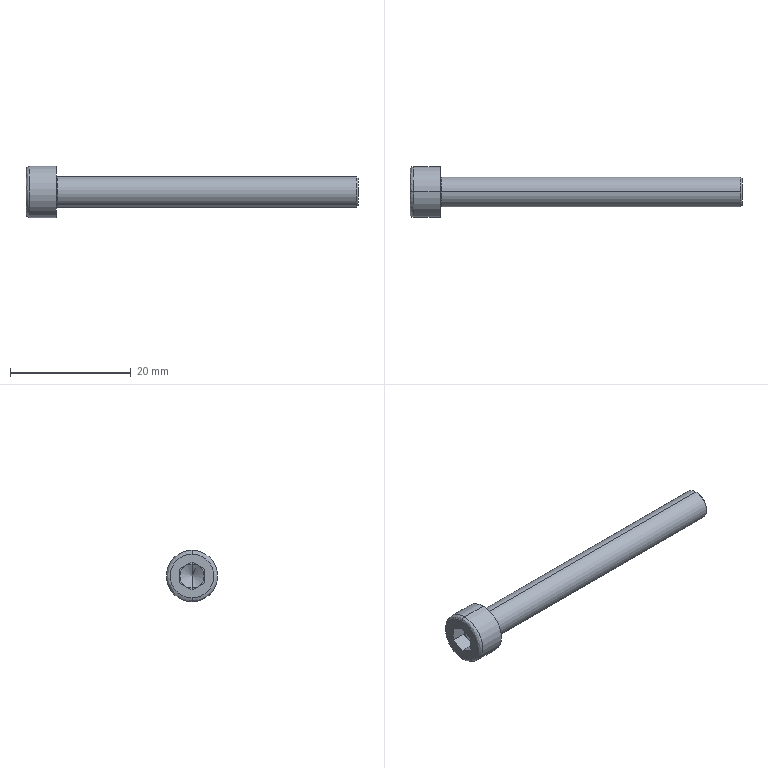Part | SolidWorks | features BaseBody 1 | 1 solid | 27 faces | box 55 x 8.5 x 8.5 mm | volume 1224 mm3 | plane 15 | spline 4 | cylinder 4 | cone 4 | commonest cylinder face diameters 5 x2 8.5 x2
STEP:
#1=CARTESIAN_POINT('',(5.,0.,2.7));
#2=VERTEX_POINT('',#1);
#3=CARTESIAN_POINT('',(5.,0.,-2.7));
#4=VERTEX_POINT('',#3);
#5=CARTESIAN_POINT('',(5.,0.,2.7));
#6=CARTESIAN_POINT('',(5.,0.1716,2.7));
#7=CARTESIAN_POINT('',(5.,0.4245,2.676));
#8=CARTESIAN_POINT('',(5.,0.7118,2.607));
#9=CARTESIAN_POINT('',(5.,0.8535,2.562));
#10=CARTESIAN_POINT('',(5.,0.9138,2.541));
#11=CARTESIAN_POINT('',(5.,0.9539,2.526));
#12=CARTESIAN_POINT('',(5.,0.9722,2.519));
#13=CARTESIAN_POINT('',(5.,1.34,2.373));
#14=CARTESIAN_POINT('',(5.,1.646,2.172));
#15=CARTESIAN_POINT('',(5.,2.041,1.778));
#16=CARTESIAN_POINT('',(5.,2.215,1.564));
#17=CARTESIAN_POINT('',(5.,2.376,1.288));
#18=CARTESIAN_POINT('',(5.,2.447,1.143));
#19=CARTESIAN_POINT('',(5.,2.475,1.08));
#20=CARTESIAN_POINT('',(5.,2.493,1.037));
#21=CARTESIAN_POINT('',(5.,2.503,1.014));
#22=CARTESIAN_POINT('',(5.,2.637,0.675));
#23=CARTESIAN_POINT('',(5.,2.7,0.343));
#24=CARTESIAN_POINT('',(5.,2.7,-0.1715));
#25=CARTESIAN_POINT('',(5.,2.676,-0.4243));
#26=CARTESIAN_POINT('',(5.,2.607,-0.7117));
#27=CARTESIAN_POINT('',(5.,2.562,-0.8534));
#28=CARTESIAN_POINT('',(5.,2.541,-0.9137));
#29=CARTESIAN_POINT('',(5.,2.526,-0.9539));
#30=CARTESIAN_POINT('',(5.,2.519,-0.9722));
#31=CARTESIAN_POINT('',(5.,2.373,-1.34));
#32=CARTESIAN_POINT('',(5.,2.172,-1.646));
#33=CARTESIAN_POINT('',(5.,1.778,-2.041));
#34=CARTESIAN_POINT('',(5.,1.564,-2.215));
#35=CARTESIAN_POINT('',(5.,1.288,-2.376));
#36=CARTESIAN_POINT('',(5.,1.143,-2.447));
#37=CARTESIAN_POINT('',(5.,1.08,-2.475));
#38=CARTESIAN_POINT('',(5.,1.037,-2.493));
#39=CARTESIAN_POINT('',(5.,1.014,-2.503));
#40=CARTESIAN_POINT('',(5.,0.6748,-2.637));
#41=CARTESIAN_POINT('',(5.,0.3435,-2.7));
#42=CARTESIAN_POINT('',(5.,0.,-2.7));
#43=B_SPLINE_CURVE_WITH_KNOTS('',3,(#5,#6,#7,#8,#9,#10,#11,#12,#13,#14,#15,#16,#17,#18,#19,#20,#21,#22,#23,#24,#25,#26,#27,#28,#29,#30,#31,#32,#33,#34,#35,#36,#37,#38,#39,#40,#41,#42),.UNSPECIFIED.,.F.,.F.,(4,1,1,1,2,2,2,1,1,1,2,2,2,1,1,1,2,2,2,1,1,1,2,2,4),(0.,0.0625,0.09375,0.1094,0.1172,0.125,0.25,0.3125,0.3437,0.3594,0.3672,0.375,0.5,0.5625,0.5937,0.6094,0.6172,0.625,0.75,0.8125,0.8437,0.8594,0.8672,0.875,1.),.UNSPECIFIED.);
#44=EDGE_CURVE('',#2,#4,#43,.T.);
#45=ORIENTED_EDGE('',*,*,#44,.F.);
#46=CARTESIAN_POINT('',(5.2,0.,2.5));
#47=VERTEX_POINT('',#46);
#48=CARTESIAN_POINT('',(5.2,0.,2.7));
#49=DIRECTION('',(0.,-1.,0.));
#50=DIRECTION('',(0.,0.,1.));
#51=AXIS2_PLACEMENT_3D('',#48,#49,#50);
#52=CIRCLE('',#51,0.2);
#53=EDGE_CURVE('',#2,#47,#52,.T.);
#54=ORIENTED_EDGE('',*,*,#53,.T.);
#55=CARTESIAN_POINT('',(5.2,0.,-2.5));
#56=VERTEX_POINT('',#55);
#57=CARTESIAN_POINT('',(5.2,0.,0.));
#58=DIRECTION('',(1.,0.,0.));
#59=DIRECTION('',(0.,0.,1.));
#60=AXIS2_PLACEMENT_3D('',#57,#58,#59);
#61=CIRCLE('',#60,2.5);
#62=EDGE_CURVE('',#56,#47,#61,.T.);
#63=ORIENTED_EDGE('',*,*,#62,.F.);
#64=CARTESIAN_POINT('',(5.2,0.,-2.7));
#65=DIRECTION('',(0.,1.,0.));
#66=DIRECTION('',(0.,0.,-1.));
#67=AXIS2_PLACEMENT_3D('',#64,#65,#66);
#68=CIRCLE('',#67,0.2);
#69=EDGE_CURVE('',#4,#56,#68,.T.);
#70=ORIENTED_EDGE('',*,*,#69,.F.);
#71=EDGE_LOOP('',(#45,#54,#63,#70));
#72=FACE_OUTER_BOUND('',#71,.T.);
#73=CARTESIAN_POINT('',(5.,0.,-2.7));
#74=CARTESIAN_POINT('',(5.,5.4,-2.7));
#75=CARTESIAN_POINT('',(5.,5.4,2.7));
#76=CARTESIAN_POINT('',(5.,0.,2.7));
#77=CARTESIAN_POINT('',(5.,0.,-2.583));
#78=CARTESIAN_POINT('',(5.,5.166,-2.583));
#79=CARTESIAN_POINT('',(5.,5.166,2.583));
#80=CARTESIAN_POINT('',(5.,0.,2.583));
#81=CARTESIAN_POINT('',(5.083,0.,-2.5));
#82=CARTESIAN_POINT('',(5.083,5.,-2.5));
#83=CARTESIAN_POINT('',(5.083,5.,2.5));
#84=CARTESIAN_POINT('',(5.083,0.,2.5));
#85=CARTESIAN_POINT('',(5.2,0.,-2.5));
#86=CARTESIAN_POINT('',(5.2,5.,-2.5));
#87=CARTESIAN_POINT('',(5.2,5.,2.5));
#88=CARTESIAN_POINT('',(5.2,0.,2.5));
#89=(BOUNDED_SURFACE()B_SPLINE_SURFACE(3,3,((#73,#74,#75,#76),(#77,#78,#79,#80),(#81,#82,#83,#84),(#85,#86,#87,#88)),.UNSPECIFIED.,.F.,.F.,.T.)B_SPLINE_SURFACE_WITH_KNOTS((4,4),(4,4),(0.,1.),(0.,1.),.UNSPECIFIED.)GEOMETRIC_REPRESENTATION_ITEM()RATIONAL_B_SPLINE_SURFACE(((1.,0.3333,0.3333,1.),(0.8047,0.2682,0.2682,0.8047),(0.8047,0.2682,0.2682,0.8047),(1.,0.3333,0.3333,1.)))REPRESENTATION_ITEM('')SURFACE());
#90=ADVANCED_FACE('',(#72),#89,.F.);
#91=CARTESIAN_POINT('',(0.625,0.,4.25));
#92=VERTEX_POINT('',#91);
#93=CARTESIAN_POINT('',(0.625,0.,-4.25));
#94=VERTEX_POINT('',#93);
#95=CARTESIAN_POINT('',(0.625,0.,0.));
#96=DIRECTION('',(1.,0.,0.));
#97=DIRECTION('',(0.,0.,1.));
#98=AXIS2_PLACEMENT_3D('',#95,#96,#97);
#99=CIRCLE('',#98,4.25);
#100=EDGE_CURVE('',#92,#94,#99,.T.);
#101=ORIENTED_EDGE('',*,*,#100,.F.);
#102=CARTESIAN_POINT('',(0.,0.,3.625));
#103=VERTEX_POINT('',#102);
#104=CARTESIAN_POINT('',(0.625,0.,3.625));
#105=DIRECTION('',(0.,-1.,0.));
#106=DIRECTION('',(0.,0.,1.));
#107=AXIS2_PLACEMENT_3D('',#104,#105,#106);
#108=CIRCLE('',#107,0.625);
#109=EDGE_CURVE('',#92,#103,#108,.T.);
#110=ORIENTED_EDGE('',*,*,#109,.T.);
#111=CARTESIAN_POINT('',(0.,0.,-3.625));
#112=VERTEX_POINT('',#111);
#113=CARTESIAN_POINT('',(0.,0.,3.625));
#114=CARTESIAN_POINT('',(0.,-7.25,3.625));
#115=CARTESIAN_POINT('',(0.,-7.25,-3.625));
#116=CARTESIAN_POINT('',(0.,0.,-3.625));
#117=(BOUNDED_CURVE()B_SPLINE_CURVE(3,(#113,#114,#115,#116),.UNSPECIFIED.,.F.,.F.)B_SPLINE_CURVE_WITH_KNOTS((4,4),(0.,1.),.UNSPECIFIED.)CURVE()GEOMETRIC_REPRESENTATION_ITEM()RATIONAL_B_SPLINE_CURVE((1.,0.3333,0.3333,1.))REPRESENTATION_ITEM(''));
#118=EDGE_CURVE('',#103,#112,#117,.T.);
#119=ORIENTED_EDGE('',*,*,#118,.T.);
#120=CARTESIAN_POINT('',(0.625,0.,-3.625));
#121=DIRECTION('',(0.,1.,0.));
#122=DIRECTION('',(0.,0.,-1.));
#123=AXIS2_PLACEMENT_3D('',#120,#121,#122);
#124=CIRCLE('',#123,0.625);
#125=EDGE_CURVE('',#94,#112,#124,.T.);
#126=ORIENTED_EDGE('',*,*,#125,.F.);
#127=EDGE_LOOP('',(#101,#110,#119,#126));
#128=FACE_OUTER_BOUND('',#127,.T.);
#129=CARTESIAN_POINT('',(0.625,0.,4.25));
#130=CARTESIAN_POINT('',(0.625,-8.5,4.25));
#131=CARTESIAN_POINT('',(0.625,-8.5,-4.25));
#132=CARTESIAN_POINT('',(0.625,0.,-4.25));
#133=CARTESIAN_POINT('',(0.2589,0.,4.25));
#134=CARTESIAN_POINT('',(0.2589,-8.5,4.25));
#135=CARTESIAN_POINT('',(0.2589,-8.5,-4.25));
#136=CARTESIAN_POINT('',(0.2589,0.,-4.25));
#137=CARTESIAN_POINT('',(0.,0.,3.991));
#138=CARTESIAN_POINT('',(0.,-7.982,3.991));
#139=CARTESIAN_POINT('',(0.,-7.982,-3.991));
#140=CARTESIAN_POINT('',(0.,0.,-3.991));
#141=CARTESIAN_POINT('',(0.,0.,3.625));
#142=CARTESIAN_POINT('',(0.,-7.25,3.625));
#143=CARTESIAN_POINT('',(0.,-7.25,-3.625));
#144=CARTESIAN_POINT('',(0.,0.,-3.625));
#145=(BOUNDED_SURFACE()B_SPLINE_SURFACE(3,3,((#129,#130,#131,#132),(#133,#134,#135,#136),(#137,#138,#139,#140),(#141,#142,#143,#144)),.UNSPECIFIED.,.F.,.F.,.F.)B_SPLINE_SURFACE_WITH_KNOTS((4,4),(4,4),(0.,1.),(0.,1.),.UNSPECIFIED.)GEOMETRIC_REPRESENTATION_ITEM()RATIONAL_B_SPLINE_SURFACE(((1.,0.3333,0.3333,1.),(0.8047,0.2682,0.2682,0.8047),(0.8047,0.2682,0.2682,0.8047),(1.,0.3333,0.3333,1.)))REPRESENTATION_ITEM('')SURFACE());
#146=ADVANCED_FACE('',(#128),#145,.T.);
#147=CARTESIAN_POINT('',(54.8,0.,2.5));
#148=VERTEX_POINT('',#147);
#149=CARTESIAN_POINT('',(54.8,0.,-2.5));
#150=VERTEX_POINT('',#149);
#151=CARTESIAN_POINT('',(54.8,0.,0.));
#152=DIRECTION('',(-1.,0.,0.));
#153=DIRECTION('',(0.,0.,1.));
#154=AXIS2_PLACEMENT_3D('',#151,#152,#153);
#155=CIRCLE('',#154,2.5);
#156=EDGE_CURVE('',#148,#150,#155,.T.);
#157=ORIENTED_EDGE('',*,*,#156,.T.);
#158=CARTESIAN_POINT('',(55.,0.,-2.5));
#159=DIRECTION('',(-1.,0.,0.));
#160=VECTOR('',#159,1000.);
#161=LINE('',#158,#160);
#162=EDGE_CURVE('',#150,#56,#161,.T.);
#163=ORIENTED_EDGE('',*,*,#162,.T.);
#164=ORIENTED_EDGE('',*,*,#62,.T.);
#165=CARTESIAN_POINT('',(55.,0.,2.5));
#166=DIRECTION('',(-1.,0.,0.));
#167=VECTOR('',#166,1000.);
#168=LINE('',#165,#167);
#169=EDGE_CURVE('',#148,#47,#168,.T.);
#170=ORIENTED_EDGE('',*,*,#169,.F.);
#171=EDGE_LOOP('',(#157,#163,#164,#170));
#172=FACE_OUTER_BOUND('',#171,.T.);
#173=CARTESIAN_POINT('',(55.,0.,0.));
#174=DIRECTION('',(-1.,0.,0.));
#175=DIRECTION('',(0.,0.,1.));
#176=AXIS2_PLACEMENT_3D('',#173,#174,#175);
#177=CYLINDRICAL_SURFACE('',#176,2.5);
#178=ADVANCED_FACE('',(#172),#177,.T.);
#179=CARTESIAN_POINT('',(55.,0.,2.3));
#180=VERTEX_POINT('',#179);
#181=CARTESIAN_POINT('',(55.,0.,-2.3));
#182=VERTEX_POINT('',#181);
#183=CARTESIAN_POINT('',(55.,0.,0.));
#184=DIRECTION('',(-1.,0.,0.));
#185=DIRECTION('',(0.,0.,1.));
#186=AXIS2_PLACEMENT_3D('',#183,#184,#185);
#187=CIRCLE('',#186,2.3);
#188=EDGE_CURVE('',#180,#182,#187,.T.);
#189=ORIENTED_EDGE('',*,*,#188,.T.);
#190=CARTESIAN_POINT('',(54.8,0.,-2.5));
#191=DIRECTION('',(-0.7071,0.,-0.7071));
#192=VECTOR('',#191,1000.);
#193=LINE('',#190,#192);
#194=EDGE_CURVE('',#182,#150,#193,.T.);
#195=ORIENTED_EDGE('',*,*,#194,.T.);
#196=ORIENTED_EDGE('',*,*,#156,.F.);
#197=CARTESIAN_POINT('',(54.8,0.,2.5));
#198=DIRECTION('',(-0.7071,0.,0.7071));
#199=VECTOR('',#198,1000.);
#200=LINE('',#197,#199);
#201=EDGE_CURVE('',#180,#148,#200,.T.);
#202=ORIENTED_EDGE('',*,*,#201,.F.);
#203=EDGE_LOOP('',(#189,#195,#196,#202));
#204=FACE_OUTER_BOUND('',#203,.T.);
#205=CARTESIAN_POINT('',(54.8,0.,0.));
#206=DIRECTION('',(-1.,0.,0.));
#207=DIRECTION('',(0.,0.,1.));
#208=AXIS2_PLACEMENT_3D('',#205,#206,#207);
#209=CONICAL_SURFACE('',#208,2.5,0.7854);
#210=ADVANCED_FACE('',(#204),#209,.T.);
#211=CARTESIAN_POINT('',(5.,0.,-4.25));
#212=VERTEX_POINT('',#211);
#213=CARTESIAN_POINT('',(5.,0.,4.25));
#214=VERTEX_POINT('',#213);
#215=CARTESIAN_POINT('',(5.,0.,0.));
#216=DIRECTION('',(1.,0.,0.));
#217=DIRECTION('',(0.,0.,1.));
#218=AXIS2_PLACEMENT_3D('',#215,#216,#217);
#219=CIRCLE('',#218,4.25);
#220=EDGE_CURVE('',#212,#214,#219,.T.);
#221=ORIENTED_EDGE('',*,*,#220,.F.);
#222=CARTESIAN_POINT('',(5.,0.,-4.25));
#223=DIRECTION('',(-1.,0.,0.));
#224=VECTOR('',#223,1000.);
#225=LINE('',#222,#224);
#226=EDGE_CURVE('',#212,#94,#225,.T.);
#227=ORIENTED_EDGE('',*,*,#226,.T.);
#228=CARTESIAN_POINT('',(0.625,0.,0.));
#229=DIRECTION('',(1.,0.,0.));
#230=DIRECTION('',(0.,0.,1.));
#231=AXIS2_PLACEMENT_3D('',#228,#229,#230);
#232=CIRCLE('',#231,4.25);
#233=EDGE_CURVE('',#94,#92,#232,.T.);
#234=ORIENTED_EDGE('',*,*,#233,.T.);
#235=CARTESIAN_POINT('',(5.,0.,4.25));
#236=DIRECTION('',(-1.,0.,0.));
#237=VECTOR('',#236,1000.);
#238=LINE('',#235,#237);
#239=EDGE_CURVE('',#214,#92,#238,.T.);
#240=ORIENTED_EDGE('',*,*,#239,.F.);
#241=EDGE_LOOP('',(#221,#227,#234,#240));
#242=FACE_OUTER_BOUND('',#241,.T.);
#243=CARTESIAN_POINT('',(5.,0.,0.));
#244=DIRECTION('',(-1.,0.,0.));
#245=DIRECTION('',(0.,0.,1.));
#246=AXIS2_PLACEMENT_3D('',#243,#244,#245);
#247=CYLINDRICAL_SURFACE('',#246,4.25);
#248=ADVANCED_FACE('',(#242),#247,.T.);
#249=CARTESIAN_POINT('',(3.655,0.,0.));
#250=VERTEX_POINT('',#249);
#251=CARTESIAN_POINT('',(2.5,0.,2.));
#252=VERTEX_POINT('',#251);
#253=CARTESIAN_POINT('',(2.5,0.,2.));
#254=DIRECTION('',(-0.5,0.,0.866));
#255=VECTOR('',#254,1000.);
#256=LINE('',#253,#255);
#257=EDGE_CURVE('',#250,#252,#256,.T.);
#258=ORIENTED_EDGE('',*,*,#257,.F.);
#259=CARTESIAN_POINT('',(2.5,0.,-2.));
#260=VERTEX_POINT('',#259);
#261=CARTESIAN_POINT('',(2.5,0.,-2.));
#262=DIRECTION('',(-0.5,0.,-0.866));
#263=VECTOR('',#262,1000.);
#264=LINE('',#261,#263);
#265=EDGE_CURVE('',#250,#260,#264,.T.);
#266=ORIENTED_EDGE('',*,*,#265,.T.);
#267=CARTESIAN_POINT('',(2.5,-1.,-1.732));
#268=VERTEX_POINT('',#267);
#269=CARTESIAN_POINT('',(2.5,0.,0.));
#270=DIRECTION('',(1.,0.,0.));
#271=DIRECTION('',(0.,0.,1.));
#272=AXIS2_PLACEMENT_3D('',#269,#270,#271);
#273=CIRCLE('',#272,2.);
#274=EDGE_CURVE('',#268,#260,#273,.T.);
#275=ORIENTED_EDGE('',*,*,#274,.F.);
#276=CARTESIAN_POINT('',(2.5,-2.,0.));
#277=VERTEX_POINT('',#276);
#278=CARTESIAN_POINT('',(2.5,0.,0.));
#279=DIRECTION('',(-1.,0.,0.));
#280=DIRECTION('',(0.,0.,1.));
#281=AXIS2_PLACEMENT_3D('',#278,#279,#280);
#282=CIRCLE('',#281,2.);
#283=EDGE_CURVE('',#268,#277,#282,.T.);
#284=ORIENTED_EDGE('',*,*,#283,.T.);
#285=CARTESIAN_POINT('',(2.5,-1.,1.732));
#286=VERTEX_POINT('',#285);
#287=CARTESIAN_POINT('',(2.5,0.,0.));
#288=DIRECTION('',(1.,0.,0.));
#289=DIRECTION('',(0.,0.,1.));
#290=AXIS2_PLACEMENT_3D('',#287,#288,#289);
#291=CIRCLE('',#290,2.);
#292=EDGE_CURVE('',#286,#277,#291,.T.);
#293=ORIENTED_EDGE('',*,*,#292,.F.);
#294=CARTESIAN_POINT('',(2.5,0.,0.));
#295=DIRECTION('',(1.,0.,0.));
#296=DIRECTION('',(0.,0.,1.));
#297=AXIS2_PLACEMENT_3D('',#294,#295,#296);
#298=CIRCLE('',#297,2.);
#299=EDGE_CURVE('',#252,#286,#298,.T.);
#300=ORIENTED_EDGE('',*,*,#299,.F.);
#301=EDGE_LOOP('',(#258,#266,#275,#284,#293,#300));
#302=FACE_OUTER_BOUND('',#301,.T.);
#303=CARTESIAN_POINT('',(2.5,0.,0.));
#304=DIRECTION('',(-1.,0.,0.));
#305=DIRECTION('',(0.,0.,1.));
#306=AXIS2_PLACEMENT_3D('',#303,#304,#305);
#307=CONICAL_SURFACE('',#306,2.,1.047);
#308=ADVANCED_FACE('',(#302),#307,.F.);
#309=ORIENTED_EDGE('',*,*,#162,.F.);
#310=CARTESIAN_POINT('',(54.8,0.,0.));
#311=DIRECTION('',(-1.,0.,0.));
#312=DIRECTION('',(0.,0.,1.));
#313=AXIS2_PLACEMENT_3D('',#310,#311,#312);
#314=CIRCLE('',#313,2.5);
#315=EDGE_CURVE('',#150,#148,#314,.T.);
#316=ORIENTED_EDGE('',*,*,#315,.T.);
#317=ORIENTED_EDGE('',*,*,#169,.T.);
#318=CARTESIAN_POINT('',(5.2,0.,0.));
#319=DIRECTION('',(1.,0.,0.));
#320=DIRECTION('',(0.,0.,1.));
#321=AXIS2_PLACEMENT_3D('',#318,#319,#320);
#322=CIRCLE('',#321,2.5);
#323=EDGE_CURVE('',#47,#56,#322,.T.);
#324=ORIENTED_EDGE('',*,*,#323,.T.);
#325=EDGE_LOOP('',(#309,#316,#317,#324));
#326=FACE_OUTER_BOUND('',#325,.T.);
#327=CARTESIAN_POINT('',(55.,0.,0.));
#328=DIRECTION('',(-1.,0.,0.));
#329=DIRECTION('',(0.,0.,1.));
#330=AXIS2_PLACEMENT_3D('',#327,#328,#329);
#331=CYLINDRICAL_SURFACE('',#330,2.5);
#332=ADVANCED_FACE('',(#326),#331,.T.);
#333=ORIENTED_EDGE('',*,*,#53,.F.);
#334=CARTESIAN_POINT('',(5.,0.,-2.7));
#335=CARTESIAN_POINT('',(5.,-0.1716,-2.7));
#336=CARTESIAN_POINT('',(5.,-0.4245,-2.676));
#337=CARTESIAN_POINT('',(5.,-0.7118,-2.607));
#338=CARTESIAN_POINT('',(5.,-0.8535,-2.562));
#339=CARTESIAN_POINT('',(5.,-0.9138,-2.541));
#340=CARTESIAN_POINT('',(5.,-0.9539,-2.526));
#341=CARTESIAN_POINT('',(5.,-0.9722,-2.519));
#342=CARTESIAN_POINT('',(5.,-1.34,-2.373));
#343=CARTESIAN_POINT('',(5.,-1.646,-2.172));
#344=CARTESIAN_POINT('',(5.,-2.041,-1.778));
#345=CARTESIAN_POINT('',(5.,-2.215,-1.564));
#346=CARTESIAN_POINT('',(5.,-2.376,-1.288));
#347=CARTESIAN_POINT('',(5.,-2.447,-1.143));
#348=CARTESIAN_POINT('',(5.,-2.475,-1.08));
#349=CARTESIAN_POINT('',(5.,-2.493,-1.037));
#350=CARTESIAN_POINT('',(5.,-2.503,-1.014));
#351=CARTESIAN_POINT('',(5.,-2.637,-0.675));
#352=CARTESIAN_POINT('',(5.,-2.7,-0.343));
#353=CARTESIAN_POINT('',(5.,-2.7,0.1715));
#354=CARTESIAN_POINT('',(5.,-2.676,0.4243));
#355=CARTESIAN_POINT('',(5.,-2.607,0.7117));
#356=CARTESIAN_POINT('',(5.,-2.562,0.8534));
#357=CARTESIAN_POINT('',(5.,-2.541,0.9137));
#358=CARTESIAN_POINT('',(5.,-2.526,0.9539));
#359=CARTESIAN_POINT('',(5.,-2.519,0.9722));
#360=CARTESIAN_POINT('',(5.,-2.373,1.34));
#361=CARTESIAN_POINT('',(5.,-2.172,1.646));
#362=CARTESIAN_POINT('',(5.,-1.778,2.041));
#363=CARTESIAN_POINT('',(5.,-1.564,2.215));
#364=CARTESIAN_POINT('',(5.,-1.288,2.376));
#365=CARTESIAN_POINT('',(5.,-1.143,2.447));
#366=CARTESIAN_POINT('',(5.,-1.08,2.475));
#367=CARTESIAN_POINT('',(5.,-1.037,2.493));
#368=CARTESIAN_POINT('',(5.,-1.014,2.503));
#369=CARTESIAN_POINT('',(5.,-0.6748,2.637));
#370=CARTESIAN_POINT('',(5.,-0.3435,2.7));
#371=CARTESIAN_POINT('',(5.,0.,2.7));
#372=B_SPLINE_CURVE_WITH_KNOTS('',3,(#334,#335,#336,#337,#338,#339,#340,#341,#342,#343,#344,#345,#346,#347,#348,#349,#350,#351,#352,#353,#354,#355,#356,#357,#358,#359,#360,#361,#362,#363,#364,#365,#366,#367,#368,#369,#370,#371),.UNSPECIFIED.,.F.,.F.,(4,1,1,1,2,2,2,1,1,1,2,2,2,1,1,1,2,2,2,1,1,1,2,2,4),(0.,0.0625,0.09375,0.1094,0.1172,0.125,0.25,0.3125,0.3437,0.3594,0.3672,0.375,0.5,0.5625,0.5937,0.6094,0.6172,0.625,0.75,0.8125,0.8437,0.8594,0.8672,0.875,1.),.UNSPECIFIED.);
#373=EDGE_CURVE('',#4,#2,#372,.T.);
#374=ORIENTED_EDGE('',*,*,#373,.F.);
#375=ORIENTED_EDGE('',*,*,#69,.T.);
#376=ORIENTED_EDGE('',*,*,#323,.F.);
#377=EDGE_LOOP('',(#333,#374,#375,#376));
#378=FACE_OUTER_BOUND('',#377,.T.);
#379=CARTESIAN_POINT('',(5.,0.,2.7));
#380=CARTESIAN_POINT('',(5.,-5.4,2.7));
#381=CARTESIAN_POINT('',(5.,-5.4,-2.7));
#382=CARTESIAN_POINT('',(5.,0.,-2.7));
#383=CARTESIAN_POINT('',(5.,0.,2.583));
#384=CARTESIAN_POINT('',(5.,-5.166,2.583));
#385=CARTESIAN_POINT('',(5.,-5.166,-2.583));
#386=CARTESIAN_POINT('',(5.,0.,-2.583));
#387=CARTESIAN_POINT('',(5.083,0.,2.5));
#388=CARTESIAN_POINT('',(5.083,-5.,2.5));
#389=CARTESIAN_POINT('',(5.083,-5.,-2.5));
#390=CARTESIAN_POINT('',(5.083,0.,-2.5));
#391=CARTESIAN_POINT('',(5.2,0.,2.5));
#392=CARTESIAN_POINT('',(5.2,-5.,2.5));
#393=CARTESIAN_POINT('',(5.2,-5.,-2.5));
#394=CARTESIAN_POINT('',(5.2,0.,-2.5));
#395=(BOUNDED_SURFACE()B_SPLINE_SURFACE(3,3,((#379,#380,#381,#382),(#383,#384,#385,#386),(#387,#388,#389,#390),(#391,#392,#393,#394)),.UNSPECIFIED.,.F.,.F.,.F.)B_SPLINE_SURFACE_WITH_KNOTS((4,4),(4,4),(0.,1.),(0.,1.),.UNSPECIFIED.)GEOMETRIC_REPRESENTATION_ITEM()RATIONAL_B_SPLINE_SURFACE(((1.,0.3333,0.3333,1.),(0.8047,0.2682,0.2682,0.8047),(0.8047,0.2682,0.2682,0.8047),(1.,0.3333,0.3333,1.)))REPRESENTATION_ITEM('')SURFACE());
#396=ADVANCED_FACE('',(#378),#395,.F.);
#397=ORIENTED_EDGE('',*,*,#194,.F.);
#398=CARTESIAN_POINT('',(55.,0.,0.));
#399=DIRECTION('',(-1.,0.,0.));
#400=DIRECTION('',(0.,0.,1.));
#401=AXIS2_PLACEMENT_3D('',#398,#399,#400);
#402=CIRCLE('',#401,2.3);
#403=EDGE_CURVE('',#182,#180,#402,.T.);
#404=ORIENTED_EDGE('',*,*,#403,.T.);
#405=ORIENTED_EDGE('',*,*,#201,.T.);
#406=ORIENTED_EDGE('',*,*,#315,.F.);
#407=EDGE_LOOP('',(#397,#404,#405,#406));
#408=FACE_OUTER_BOUND('',#407,.T.);
#409=CARTESIAN_POINT('',(54.8,0.,0.));
#410=DIRECTION('',(-1.,0.,0.));
#411=DIRECTION('',(0.,0.,1.));
#412=AXIS2_PLACEMENT_3D('',#409,#410,#411);
#413=CONICAL_SURFACE('',#412,2.5,0.7854);
#414=ADVANCED_FACE('',(#408),#413,.T.);
#415=CARTESIAN_POINT('',(5.,0.,0.));
#416=DIRECTION('',(1.,0.,0.));
#417=DIRECTION('',(0.,0.,1.));
#418=AXIS2_PLACEMENT_3D('',#415,#416,#417);
#419=CIRCLE('',#418,4.25);
#420=EDGE_CURVE('',#214,#212,#419,.T.);
#421=ORIENTED_EDGE('',*,*,#420,.T.);
#422=ORIENTED_EDGE('',*,*,#220,.T.);
#423=EDGE_LOOP('',(#421,#422));
#424=FACE_OUTER_BOUND('',#423,.T.);
#425=ORIENTED_EDGE('',*,*,#373,.T.);
#426=ORIENTED_EDGE('',*,*,#44,.T.);
#427=EDGE_LOOP('',(#425,#426));
#428=FACE_BOUND('',#427,.T.);
#429=CARTESIAN_POINT('',(5.,0.,0.));
#430=DIRECTION('',(1.,0.,0.));
#431=DIRECTION('',(0.,0.,-1.));
#432=AXIS2_PLACEMENT_3D('',#429,#430,#431);
#433=PLANE('',#432);
#434=ADVANCED_FACE('',(#424,#428),#433,.T.);
#435=ORIENTED_EDGE('',*,*,#188,.F.);
#436=ORIENTED_EDGE('',*,*,#403,.F.);
#437=EDGE_LOOP('',(#435,#436));
#438=FACE_OUTER_BOUND('',#437,.T.);
#439=CARTESIAN_POINT('',(55.,0.,0.));
#440=DIRECTION('',(1.,0.,0.));
#441=DIRECTION('',(0.,0.,-1.));
#442=AXIS2_PLACEMENT_3D('',#439,#440,#441);
#443=PLANE('',#442);
#444=ADVANCED_FACE('',(#438),#443,.T.);
#445=ORIENTED_EDGE('',*,*,#226,.F.);
#446=ORIENTED_EDGE('',*,*,#420,.F.);
#447=ORIENTED_EDGE('',*,*,#239,.T.);
#448=ORIENTED_EDGE('',*,*,#100,.T.);
#449=EDGE_LOOP('',(#445,#446,#447,#448));
#450=FACE_OUTER_BOUND('',#449,.T.);
#451=CARTESIAN_POINT('',(5.,0.,0.));
#452=DIRECTION('',(-1.,0.,0.));
#453=DIRECTION('',(0.,0.,1.));
#454=AXIS2_PLACEMENT_3D('',#451,#452,#453);
#455=CYLINDRICAL_SURFACE('',#454,4.25);
#456=ADVANCED_FACE('',(#450),#455,.T.);
#457=ORIENTED_EDGE('',*,*,#109,.F.);
#458=ORIENTED_EDGE('',*,*,#233,.F.);
#459=ORIENTED_EDGE('',*,*,#125,.T.);
#460=CARTESIAN_POINT('',(0.,0.,-3.625));
#461=CARTESIAN_POINT('',(0.,7.25,-3.625));
#462=CARTESIAN_POINT('',(0.,7.25,3.625));
#463=CARTESIAN_POINT('',(0.,0.,3.625));
#464=(BOUNDED_CURVE()B_SPLINE_CURVE(3,(#460,#461,#462,#463),.UNSPECIFIED.,.F.,.F.)B_SPLINE_CURVE_WITH_KNOTS((4,4),(0.,1.),.UNSPECIFIED.)CURVE()GEOMETRIC_REPRESENTATION_ITEM()RATIONAL_B_SPLINE_CURVE((1.,0.3333,0.3333,1.))REPRESENTATION_ITEM(''));
#465=EDGE_CURVE('',#112,#103,#464,.T.);
#466=ORIENTED_EDGE('',*,*,#465,.T.);
#467=EDGE_LOOP('',(#457,#458,#459,#466));
#468=FACE_OUTER_BOUND('',#467,.T.);
#469=CARTESIAN_POINT('',(0.625,0.,-4.25));
#470=CARTESIAN_POINT('',(0.625,8.5,-4.25));
#471=CARTESIAN_POINT('',(0.625,8.5,4.25));
#472=CARTESIAN_POINT('',(0.625,0.,4.25));
#473=CARTESIAN_POINT('',(0.2589,0.,-4.25));
#474=CARTESIAN_POINT('',(0.2589,8.5,-4.25));
#475=CARTESIAN_POINT('',(0.2589,8.5,4.25));
#476=CARTESIAN_POINT('',(0.2589,0.,4.25));
#477=CARTESIAN_POINT('',(0.,0.,-3.991));
#478=CARTESIAN_POINT('',(0.,7.982,-3.991));
#479=CARTESIAN_POINT('',(0.,7.982,3.991));
#480=CARTESIAN_POINT('',(0.,0.,3.991));
#481=CARTESIAN_POINT('',(0.,0.,-3.625));
#482=CARTESIAN_POINT('',(0.,7.25,-3.625));
#483=CARTESIAN_POINT('',(0.,7.25,3.625));
#484=CARTESIAN_POINT('',(0.,0.,3.625));
#485=(BOUNDED_SURFACE()B_SPLINE_SURFACE(3,3,((#469,#470,#471,#472),(#473,#474,#475,#476),(#477,#478,#479,#480),(#481,#482,#483,#484)),.UNSPECIFIED.,.F.,.F.,.T.)B_SPLINE_SURFACE_WITH_KNOTS((4,4),(4,4),(0.,1.),(0.,1.),.UNSPECIFIED.)GEOMETRIC_REPRESENTATION_ITEM()RATIONAL_B_SPLINE_SURFACE(((1.,0.3333,0.3333,1.),(0.8047,0.2682,0.2682,0.8047),(0.8047,0.2682,0.2682,0.8047),(1.,0.3333,0.3333,1.)))REPRESENTATION_ITEM('')SURFACE());
#486=ADVANCED_FACE('',(#468),#485,.T.);
#487=CARTESIAN_POINT('',(0.,2.,1.155));
#488=VERTEX_POINT('',#487);
#489=CARTESIAN_POINT('',(0.,2.,-1.155));
#490=VERTEX_POINT('',#489);
#491=CARTESIAN_POINT('',(0.,2.,0.));
#492=DIRECTION('',(0.,0.,-1.));
#493=VECTOR('',#492,1000.);
#494=LINE('',#491,#493);
#495=EDGE_CURVE('',#488,#490,#494,.T.);
#496=ORIENTED_EDGE('',*,*,#495,.F.);
#497=CARTESIAN_POINT('',(0.,0.,2.309));
#498=VERTEX_POINT('',#497);
#499=CARTESIAN_POINT('',(0.,0.,2.309));
#500=DIRECTION('',(0.,0.866,-0.5));
#501=VECTOR('',#500,1000.);
#502=LINE('',#499,#501);
#503=EDGE_CURVE('',#498,#488,#502,.T.);
#504=ORIENTED_EDGE('',*,*,#503,.F.);
#505=CARTESIAN_POINT('',(0.,-2.,1.155));
#506=VERTEX_POINT('',#505);
#507=CARTESIAN_POINT('',(0.,-2.,1.155));
#508=DIRECTION('',(0.,0.866,0.5));
#509=VECTOR('',#508,1000.);
#510=LINE('',#507,#509);
#511=EDGE_CURVE('',#506,#498,#510,.T.);
#512=ORIENTED_EDGE('',*,*,#511,.F.);
#513=CARTESIAN_POINT('',(0.,-2.,-1.155));
#514=VERTEX_POINT('',#513);
#515=CARTESIAN_POINT('',(0.,-2.,0.));
#516=DIRECTION('',(0.,0.,1.));
#517=VECTOR('',#516,1000.);
#518=LINE('',#515,#517);
#519=EDGE_CURVE('',#514,#506,#518,.T.);
#520=ORIENTED_EDGE('',*,*,#519,.F.);
#521=CARTESIAN_POINT('',(0.,0.,-2.309));
#522=VERTEX_POINT('',#521);
#523=CARTESIAN_POINT('',(0.,0.,-2.309));
#524=DIRECTION('',(0.,-0.866,0.5));
#525=VECTOR('',#524,1000.);
#526=LINE('',#523,#525);
#527=EDGE_CURVE('',#522,#514,#526,.T.);
#528=ORIENTED_EDGE('',*,*,#527,.F.);
#529=CARTESIAN_POINT('',(0.,2.,-1.155));
#530=DIRECTION('',(0.,-0.866,-0.5));
#531=VECTOR('',#530,1000.);
#532=LINE('',#529,#531);
#533=EDGE_CURVE('',#490,#522,#532,.T.);
#534=ORIENTED_EDGE('',*,*,#533,.F.);
#535=EDGE_LOOP('',(#496,#504,#512,#520,#528,#534));
#536=FACE_BOUND('',#535,.T.);
#537=ORIENTED_EDGE('',*,*,#465,.F.);
#538=ORIENTED_EDGE('',*,*,#118,.F.);
#539=EDGE_LOOP('',(#537,#538));
#540=FACE_OUTER_BOUND('',#539,.T.);
#541=CARTESIAN_POINT('',(0.,0.,0.));
#542=DIRECTION('',(1.,0.,0.));
#543=DIRECTION('',(0.,0.,-1.));
#544=AXIS2_PLACEMENT_3D('',#541,#542,#543);
#545=PLANE('',#544);
#546=ADVANCED_FACE('',(#536,#540),#545,.F.);
#547=CARTESIAN_POINT('',(2.5,0.,-2.309));
#548=VERTEX_POINT('',#547);
#549=CARTESIAN_POINT('',(2.5,0.,-2.309));
#550=DIRECTION('',(1.,0.,0.));
#551=VECTOR('',#550,1000.);
#552=LINE('',#549,#551);
#553=EDGE_CURVE('',#522,#548,#552,.T.);
#554=ORIENTED_EDGE('',*,*,#553,.T.);
#555=CARTESIAN_POINT('',(2.5,1.,-1.732));
#556=VERTEX_POINT('',#555);
#557=CARTESIAN_POINT('',(2.5,0.,-2.309));
#558=DIRECTION('',(0.,0.866,0.5));
#559=VECTOR('',#558,1000.);
#560=LINE('',#557,#559);
#561=EDGE_CURVE('',#548,#556,#560,.T.);
#562=ORIENTED_EDGE('',*,*,#561,.T.);
#563=CARTESIAN_POINT('',(2.5,2.,-1.155));
#564=VERTEX_POINT('',#563);
#565=CARTESIAN_POINT('',(2.5,1.,-1.732));
#566=DIRECTION('',(0.,0.866,0.5));
#567=VECTOR('',#566,1000.);
#568=LINE('',#565,#567);
#569=EDGE_CURVE('',#556,#564,#568,.T.);
#570=ORIENTED_EDGE('',*,*,#569,.T.);
#571=CARTESIAN_POINT('',(2.5,2.,-1.155));
#572=DIRECTION('',(-1.,0.,0.));
#573=VECTOR('',#572,1000.);
#574=LINE('',#571,#573);
#575=EDGE_CURVE('',#564,#490,#574,.T.);
#576=ORIENTED_EDGE('',*,*,#575,.T.);
#577=ORIENTED_EDGE('',*,*,#533,.T.);
#578=EDGE_LOOP('',(#554,#562,#570,#576,#577));
#579=FACE_OUTER_BOUND('',#578,.T.);
#580=CARTESIAN_POINT('',(2.5,0.,-2.309));
#581=DIRECTION('',(0.,-0.5,0.866));
#582=DIRECTION('',(0.,-0.866,-0.5));
#583=AXIS2_PLACEMENT_3D('',#580,#581,#582);
#584=PLANE('',#583);
#585=ADVANCED_FACE('',(#579),#584,.T.);
#586=ORIENTED_EDGE('',*,*,#575,.F.);
#587=CARTESIAN_POINT('',(2.5,2.,0.));
#588=VERTEX_POINT('',#587);
#589=CARTESIAN_POINT('',(2.5,2.,-2.309));
#590=DIRECTION('',(0.,0.,1.));
#591=VECTOR('',#590,1000.);
#592=LINE('',#589,#591);
#593=EDGE_CURVE('',#564,#588,#592,.T.);
#594=ORIENTED_EDGE('',*,*,#593,.T.);
#595=CARTESIAN_POINT('',(2.5,2.,1.155));
#596=VERTEX_POINT('',#595);
#597=CARTESIAN_POINT('',(2.5,2.,-2.309));
#598=DIRECTION('',(0.,0.,1.));
#599=VECTOR('',#598,1000.);
#600=LINE('',#597,#599);
#601=EDGE_CURVE('',#588,#596,#600,.T.);
#602=ORIENTED_EDGE('',*,*,#601,.T.);
#603=CARTESIAN_POINT('',(2.5,2.,1.155));
#604=DIRECTION('',(-1.,0.,0.));
#605=VECTOR('',#604,1000.);
#606=LINE('',#603,#605);
#607=EDGE_CURVE('',#596,#488,#606,.T.);
#608=ORIENTED_EDGE('',*,*,#607,.T.);
#609=ORIENTED_EDGE('',*,*,#495,.T.);
#610=EDGE_LOOP('',(#586,#594,#602,#608,#609));
#611=FACE_OUTER_BOUND('',#610,.T.);
#612=CARTESIAN_POINT('',(2.5,2.,-1.155));
#613=DIRECTION('',(0.,-1.,0.));
#614=DIRECTION('',(0.,0.,-1.));
#615=AXIS2_PLACEMENT_3D('',#612,#613,#614);
#616=PLANE('',#615);
#617=ADVANCED_FACE('',(#611),#616,.T.);
#618=ORIENTED_EDGE('',*,*,#607,.F.);
#619=CARTESIAN_POINT('',(2.5,1.,1.732));
#620=VERTEX_POINT('',#619);
#621=CARTESIAN_POINT('',(2.5,2.,1.155));
#622=DIRECTION('',(0.,-0.866,0.5));
#623=VECTOR('',#622,1000.);
#624=LINE('',#621,#623);
#625=EDGE_CURVE('',#596,#620,#624,.T.);
#626=ORIENTED_EDGE('',*,*,#625,.T.);
#627=CARTESIAN_POINT('',(2.5,0.,2.309));
#628=VERTEX_POINT('',#627);
#629=CARTESIAN_POINT('',(2.5,2.,1.155));
#630=DIRECTION('',(0.,-0.866,0.5));
#631=VECTOR('',#630,1000.);
#632=LINE('',#629,#631);
#633=EDGE_CURVE('',#620,#628,#632,.T.);
#634=ORIENTED_EDGE('',*,*,#633,.T.);
#635=CARTESIAN_POINT('',(2.5,0.,2.309));
#636=DIRECTION('',(-1.,0.,0.));
#637=VECTOR('',#636,1000.);
#638=LINE('',#635,#637);
#639=EDGE_CURVE('',#628,#498,#638,.T.);
#640=ORIENTED_EDGE('',*,*,#639,.T.);
#641=ORIENTED_EDGE('',*,*,#503,.T.);
#642=EDGE_LOOP('',(#618,#626,#634,#640,#641));
#643=FACE_OUTER_BOUND('',#642,.T.);
#644=CARTESIAN_POINT('',(2.5,2.,1.155));
#645=DIRECTION('',(0.,-0.5,-0.866));
#646=DIRECTION('',(0.,0.866,-0.5));
#647=AXIS2_PLACEMENT_3D('',#644,#645,#646);
#648=PLANE('',#647);
#649=ADVANCED_FACE('',(#643),#648,.T.);
#650=ORIENTED_EDGE('',*,*,#639,.F.);
#651=CARTESIAN_POINT('',(2.5,0.,2.309));
#652=DIRECTION('',(0.,-0.866,-0.5));
#653=VECTOR('',#652,1000.);
#654=LINE('',#651,#653);
#655=EDGE_CURVE('',#628,#286,#654,.T.);
#656=ORIENTED_EDGE('',*,*,#655,.T.);
#657=CARTESIAN_POINT('',(2.5,-2.,1.155));
#658=VERTEX_POINT('',#657);
#659=CARTESIAN_POINT('',(2.5,-1.,1.732));
#660=DIRECTION('',(0.,-0.866,-0.5));
#661=VECTOR('',#660,1000.);
#662=LINE('',#659,#661);
#663=EDGE_CURVE('',#286,#658,#662,.T.);
#664=ORIENTED_EDGE('',*,*,#663,.T.);
#665=CARTESIAN_POINT('',(2.5,-2.,1.155));
#666=DIRECTION('',(-1.,0.,0.));
#667=VECTOR('',#666,1000.);
#668=LINE('',#665,#667);
#669=EDGE_CURVE('',#658,#506,#668,.T.);
#670=ORIENTED_EDGE('',*,*,#669,.T.);
#671=ORIENTED_EDGE('',*,*,#511,.T.);
#672=EDGE_LOOP('',(#650,#656,#664,#670,#671));
#673=FACE_OUTER_BOUND('',#672,.T.);
#674=CARTESIAN_POINT('',(2.5,0.,2.309));
#675=DIRECTION('',(0.,0.5,-0.866));
#676=DIRECTION('',(0.,0.866,0.5));
#677=AXIS2_PLACEMENT_3D('',#674,#675,#676);
#678=PLANE('',#677);
#679=ADVANCED_FACE('',(#673),#678,.T.);
#680=ORIENTED_EDGE('',*,*,#669,.F.);
#681=CARTESIAN_POINT('',(2.5,-2.,-2.309));
#682=DIRECTION('',(0.,0.,-1.));
#683=VECTOR('',#682,1000.);
#684=LINE('',#681,#683);
#685=EDGE_CURVE('',#658,#277,#684,.T.);
#686=ORIENTED_EDGE('',*,*,#685,.T.);
#687=CARTESIAN_POINT('',(2.5,-2.,-1.155));
#688=VERTEX_POINT('',#687);
#689=CARTESIAN_POINT('',(2.5,-2.,1.155));
#690=DIRECTION('',(0.,0.,-1.));
#691=VECTOR('',#690,1000.);
#692=LINE('',#689,#691);
#693=EDGE_CURVE('',#277,#688,#692,.T.);
#694=ORIENTED_EDGE('',*,*,#693,.T.);
#695=CARTESIAN_POINT('',(2.5,-2.,-1.155));
#696=DIRECTION('',(-1.,0.,0.));
#697=VECTOR('',#696,1000.);
#698=LINE('',#695,#697);
#699=EDGE_CURVE('',#688,#514,#698,.T.);
#700=ORIENTED_EDGE('',*,*,#699,.T.);
#701=ORIENTED_EDGE('',*,*,#519,.T.);
#702=EDGE_LOOP('',(#680,#686,#694,#700,#701));
#703=FACE_OUTER_BOUND('',#702,.T.);
#704=CARTESIAN_POINT('',(2.5,-2.,1.155));
#705=DIRECTION('',(0.,1.,0.));
#706=DIRECTION('',(0.,0.,1.));
#707=AXIS2_PLACEMENT_3D('',#704,#705,#706);
#708=PLANE('',#707);
#709=ADVANCED_FACE('',(#703),#708,.T.);
#710=ORIENTED_EDGE('',*,*,#699,.F.);
#711=CARTESIAN_POINT('',(2.5,-2.,-1.155));
#712=DIRECTION('',(0.,0.866,-0.5));
#713=VECTOR('',#712,1000.);
#714=LINE('',#711,#713);
#715=EDGE_CURVE('',#688,#268,#714,.T.);
#716=ORIENTED_EDGE('',*,*,#715,.T.);
#717=CARTESIAN_POINT('',(2.5,-2.,-1.155));
#718=DIRECTION('',(0.,0.866,-0.5));
#719=VECTOR('',#718,1000.);
#720=LINE('',#717,#719);
#721=EDGE_CURVE('',#268,#548,#720,.T.);
#722=ORIENTED_EDGE('',*,*,#721,.T.);
#723=ORIENTED_EDGE('',*,*,#553,.F.);
#724=ORIENTED_EDGE('',*,*,#527,.T.);
#725=EDGE_LOOP('',(#710,#716,#722,#723,#724));
#726=FACE_OUTER_BOUND('',#725,.T.);
#727=CARTESIAN_POINT('',(2.5,-2.,-1.155));
#728=DIRECTION('',(0.,0.5,0.866));
#729=DIRECTION('',(0.,-0.866,0.5));
#730=AXIS2_PLACEMENT_3D('',#727,#728,#729);
#731=PLANE('',#730);
#732=ADVANCED_FACE('',(#726),#731,.T.);
#733=ORIENTED_EDGE('',*,*,#274,.T.);
#734=CARTESIAN_POINT('',(2.5,0.,0.));
#735=DIRECTION('',(1.,0.,0.));
#736=DIRECTION('',(0.,0.,1.));
#737=AXIS2_PLACEMENT_3D('',#734,#735,#736);
#738=CIRCLE('',#737,2.);
#739=EDGE_CURVE('',#260,#556,#738,.T.);
#740=ORIENTED_EDGE('',*,*,#739,.T.);
#741=ORIENTED_EDGE('',*,*,#561,.F.);
#742=ORIENTED_EDGE('',*,*,#721,.F.);
#743=EDGE_LOOP('',(#733,#740,#741,#742));
#744=FACE_OUTER_BOUND('',#743,.T.);
#745=CARTESIAN_POINT('',(2.5,0.,-2.309));
#746=DIRECTION('',(1.,0.,0.));
#747=DIRECTION('',(0.,0.,-1.));
#748=AXIS2_PLACEMENT_3D('',#745,#746,#747);
#749=PLANE('',#748);
#750=ADVANCED_FACE('',(#744),#749,.F.);
#751=ORIENTED_EDGE('',*,*,#633,.F.);
#752=CARTESIAN_POINT('',(2.5,0.,0.));
#753=DIRECTION('',(1.,0.,0.));
#754=DIRECTION('',(0.,0.,1.));
#755=AXIS2_PLACEMENT_3D('',#752,#753,#754);
#756=CIRCLE('',#755,2.);
#757=EDGE_CURVE('',#620,#252,#756,.T.);
#758=ORIENTED_EDGE('',*,*,#757,.T.);
#759=ORIENTED_EDGE('',*,*,#299,.T.);
#760=ORIENTED_EDGE('',*,*,#655,.F.);
#761=EDGE_LOOP('',(#751,#758,#759,#760));
#762=FACE_OUTER_BOUND('',#761,.T.);
#763=CARTESIAN_POINT('',(2.5,0.,-2.309));
#764=DIRECTION('',(1.,0.,0.));
#765=DIRECTION('',(0.,0.,-1.));
#766=AXIS2_PLACEMENT_3D('',#763,#764,#765);
#767=PLANE('',#766);
#768=ADVANCED_FACE('',(#762),#767,.F.);
#769=ORIENTED_EDGE('',*,*,#715,.F.);
#770=ORIENTED_EDGE('',*,*,#693,.F.);
#771=ORIENTED_EDGE('',*,*,#283,.F.);
#772=EDGE_LOOP('',(#769,#770,#771));
#773=FACE_OUTER_BOUND('',#772,.T.);
#774=CARTESIAN_POINT('',(2.5,0.,-2.309));
#775=DIRECTION('',(1.,0.,0.));
#776=DIRECTION('',(0.,0.,-1.));
#777=AXIS2_PLACEMENT_3D('',#774,#775,#776);
#778=PLANE('',#777);
#779=ADVANCED_FACE('',(#773),#778,.F.);
#780=ORIENTED_EDGE('',*,*,#265,.F.);
#781=ORIENTED_EDGE('',*,*,#257,.T.);
#782=ORIENTED_EDGE('',*,*,#757,.F.);
#783=CARTESIAN_POINT('',(2.5,0.,0.));
#784=DIRECTION('',(1.,0.,0.));
#785=DIRECTION('',(0.,0.,1.));
#786=AXIS2_PLACEMENT_3D('',#783,#784,#785);
#787=CIRCLE('',#786,2.);
#788=EDGE_CURVE('',#588,#620,#787,.T.);
#789=ORIENTED_EDGE('',*,*,#788,.F.);
#790=CARTESIAN_POINT('',(2.5,0.,0.));
#791=DIRECTION('',(1.,0.,0.));
#792=DIRECTION('',(0.,0.,1.));
#793=AXIS2_PLACEMENT_3D('',#790,#791,#792);
#794=CIRCLE('',#793,2.);
#795=EDGE_CURVE('',#556,#588,#794,.T.);
#796=ORIENTED_EDGE('',*,*,#795,.F.);
#797=ORIENTED_EDGE('',*,*,#739,.F.);
#798=EDGE_LOOP('',(#780,#781,#782,#789,#796,#797));
#799=FACE_OUTER_BOUND('',#798,.T.);
#800=CARTESIAN_POINT('',(2.5,0.,0.));
#801=DIRECTION('',(-1.,0.,0.));
#802=DIRECTION('',(0.,0.,1.));
#803=AXIS2_PLACEMENT_3D('',#800,#801,#802);
#804=CONICAL_SURFACE('',#803,2.,1.047);
#805=ADVANCED_FACE('',(#799),#804,.F.);
#806=ORIENTED_EDGE('',*,*,#685,.F.);
#807=ORIENTED_EDGE('',*,*,#663,.F.);
#808=ORIENTED_EDGE('',*,*,#292,.T.);
#809=EDGE_LOOP('',(#806,#807,#808));
#810=FACE_OUTER_BOUND('',#809,.T.);
#811=CARTESIAN_POINT('',(2.5,0.,-2.309));
#812=DIRECTION('',(1.,0.,0.));
#813=DIRECTION('',(0.,0.,-1.));
#814=AXIS2_PLACEMENT_3D('',#811,#812,#813);
#815=PLANE('',#814);
#816=ADVANCED_FACE('',(#810),#815,.F.);
#817=ORIENTED_EDGE('',*,*,#625,.F.);
#818=ORIENTED_EDGE('',*,*,#601,.F.);
#819=ORIENTED_EDGE('',*,*,#788,.T.);
#820=EDGE_LOOP('',(#817,#818,#819));
#821=FACE_OUTER_BOUND('',#820,.T.);
#822=CARTESIAN_POINT('',(2.5,0.,-2.309));
#823=DIRECTION('',(1.,0.,0.));
#824=DIRECTION('',(0.,0.,-1.));
#825=AXIS2_PLACEMENT_3D('',#822,#823,#824);
#826=PLANE('',#825);
#827=ADVANCED_FACE('',(#821),#826,.F.);
#828=ORIENTED_EDGE('',*,*,#593,.F.);
#829=ORIENTED_EDGE('',*,*,#569,.F.);
#830=ORIENTED_EDGE('',*,*,#795,.T.);
#831=EDGE_LOOP('',(#828,#829,#830));
#832=FACE_OUTER_BOUND('',#831,.T.);
#833=CARTESIAN_POINT('',(2.5,0.,-2.309));
#834=DIRECTION('',(1.,0.,0.));
#835=DIRECTION('',(0.,0.,-1.));
#836=AXIS2_PLACEMENT_3D('',#833,#834,#835);
#837=PLANE('',#836);
#838=ADVANCED_FACE('',(#832),#837,.F.);
#839=CLOSED_SHELL('',(#90,#146,#178,#210,#248,#308,#332,#396,#414,#434,#444,#456,#486,#546,#585,#617,#649,#679,#709,#732,#750,#768,#779,#805,#816,#827,#838));
#840=MANIFOLD_SOLID_BREP('',#839);
#841=CARTESIAN_POINT('',(0.,0.,0.));
#842=DIRECTION('',(0.,0.,1.));
#843=DIRECTION('',(1.,0.,0.));
#844=AXIS2_PLACEMENT_3D('',#841,#842,#843);
#845=(LENGTH_UNIT()NAMED_UNIT(*)SI_UNIT(.MILLI.,.METRE.));
#846=UNCERTAINTY_MEASURE_WITH_UNIT(LENGTH_MEASURE(0.00001),#845,'','');
#847=(NAMED_UNIT(*)PLANE_ANGLE_UNIT()SI_UNIT($,.RADIAN.));
#848=(NAMED_UNIT(*)SI_UNIT($,.STERADIAN.)SOLID_ANGLE_UNIT());
#849=(GEOMETRIC_REPRESENTATION_CONTEXT(3)GLOBAL_UNCERTAINTY_ASSIGNED_CONTEXT((#846))GLOBAL_UNIT_ASSIGNED_CONTEXT((#845,#847,#848))REPRESENTATION_CONTEXT('',''));
#850=ADVANCED_BREP_SHAPE_REPRESENTATION('',(#840,#844),#849);